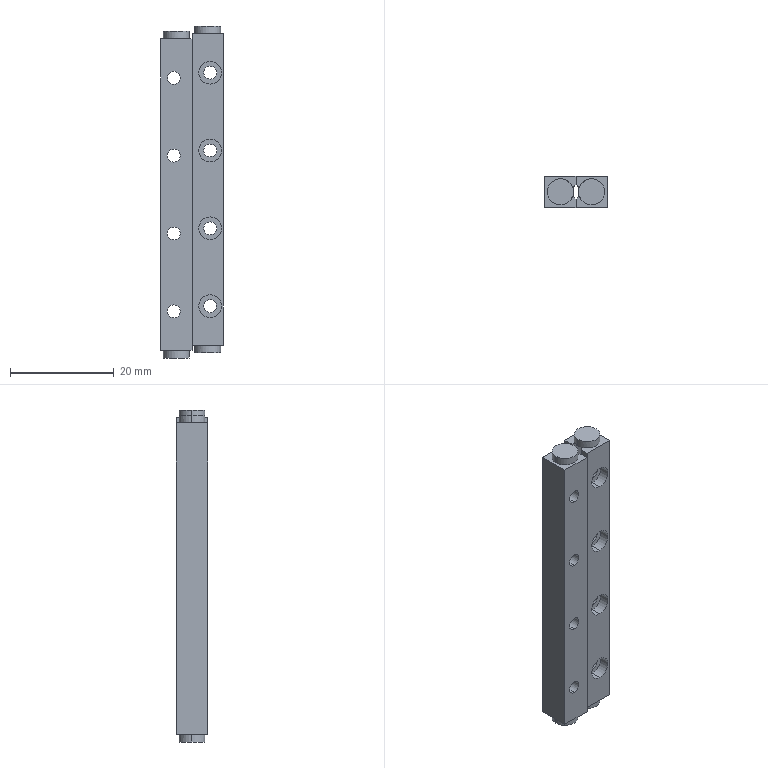Part | NX | features BREP 2 | 2 solids | 74 faces | box 12 x 6 x 64 mm | volume 3797 mm3 | cylinder 40 | plane 34 | commonest cylinder face diameters 2.5 x16 4.4 x16 5 x8